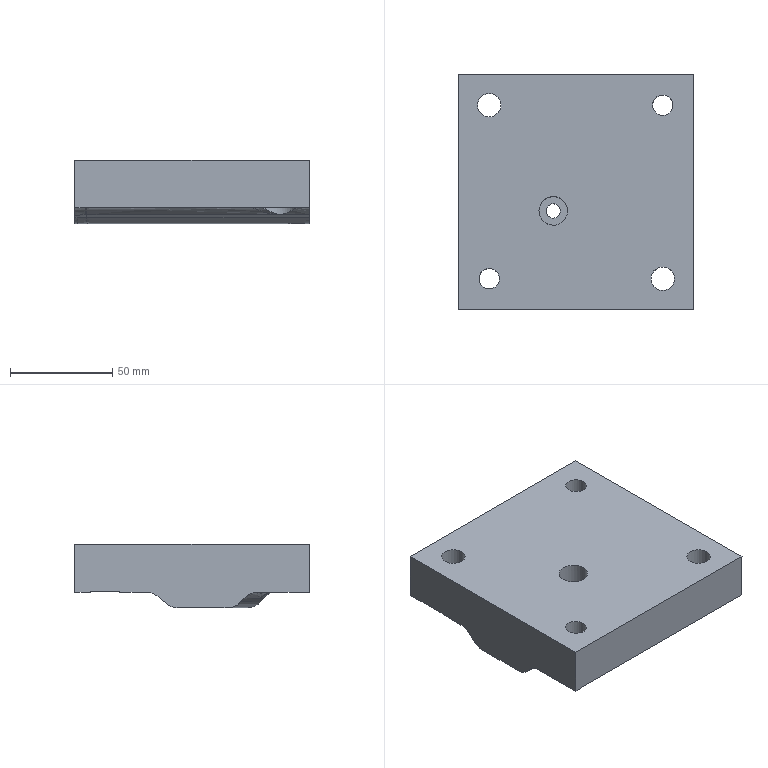Part | NX | features solid 2 | 1 solid | 62 faces | box 115.534 x 115 x 31.028 mm | volume 322840 mm3 | spline 47 | cylinder 10 | plane 5 | commonest cylinder face diameters 17.5 x5 10 x2 11.5 x2 7 x1